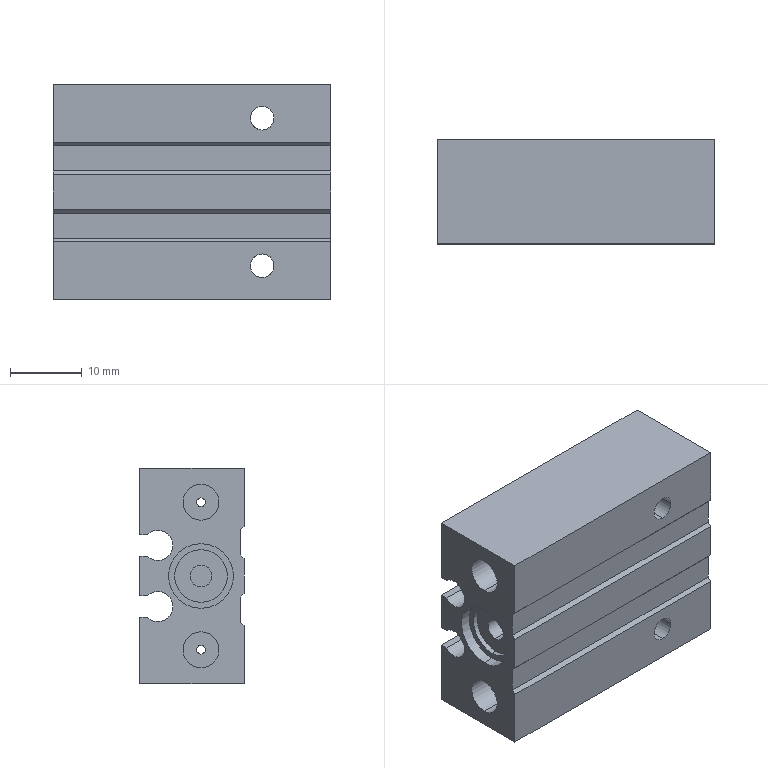Part | SolidWorks | features BaseBody 1 | 1 solid | 88 faces | box 38.5 x 14.5 x 30 mm | volume 12801 mm3 | cylinder 42 | plane 34 | cone 12 | commonest cylinder face diameters 2.459 x12 3.3 x8 6 x6 1.2 x4 5 x4 3 x2